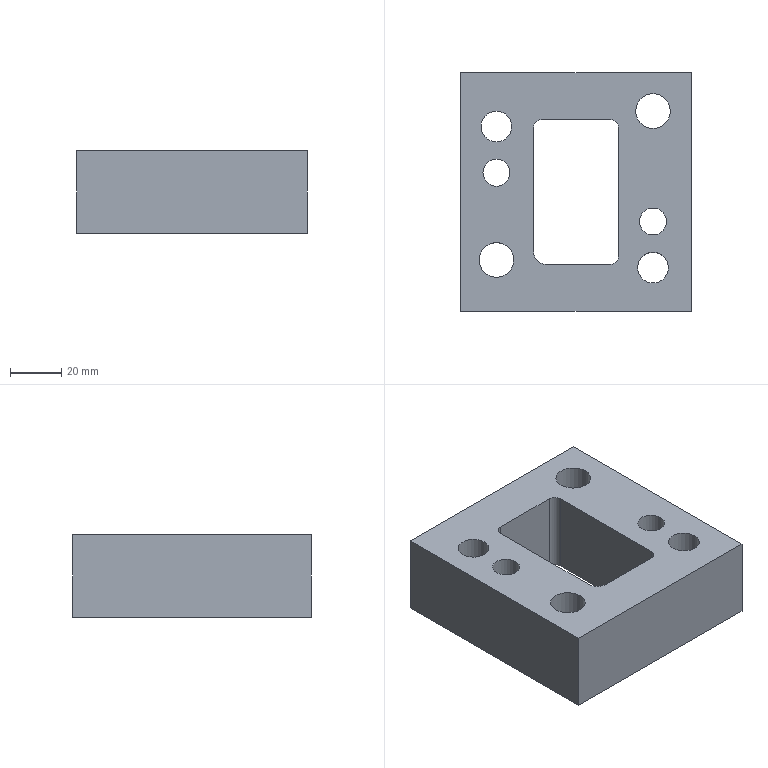Part | STEP file | lll_id2670_x_t | 1 solid | 24 faces | box 90 x 93 x 32 mm | volume 181442 mm3 | plane 12 | cylinder 12 | commonest cylinder face diameters 6 x3 10.505 x2 12 x2 13.509 x2 20.008 x2 10 x1
STEP:
#1=CARTESIAN_POINT('',(472.252,277.75,60.5));
#2=VERTEX_POINT('',#1);
#3=CARTESIAN_POINT('',(467.,277.75,60.5));
#4=DIRECTION('',(0.,0.,1.));
#5=DIRECTION('',(1.,0.,0.));
#6=AXIS2_PLACEMENT_3D('',#3,#4,#5);
#7=CIRCLE('',#6,5.253);
#8=EDGE_CURVE('',#2,#2,#7,.T.);
#9=ORIENTED_EDGE('',*,*,#8,.T.);
#10=EDGE_LOOP('',(#9));
#11=FACE_BOUND('',#10,.T.);
#12=CARTESIAN_POINT('',(395.996,262.75,60.5));
#13=VERTEX_POINT('',#12);
#14=CARTESIAN_POINT('',(406.,262.75,60.5));
#15=DIRECTION('',(0.,0.,1.));
#16=DIRECTION('',(-1.,0.,0.));
#17=AXIS2_PLACEMENT_3D('',#14,#15,#16);
#18=CIRCLE('',#17,10.004);
#19=EDGE_CURVE('',#13,#13,#18,.T.);
#20=ORIENTED_EDGE('',*,*,#19,.T.);
#21=EDGE_LOOP('',(#20));
#22=FACE_BOUND('',#21,.T.);
#23=CARTESIAN_POINT('',(420.5,314.5,60.5));
#24=VERTEX_POINT('',#23);
#25=CARTESIAN_POINT('',(420.5,266.,60.5));
#26=VERTEX_POINT('',#25);
#27=CARTESIAN_POINT('',(420.5,300.,60.5));
#28=DIRECTION('',(0.,-1.,0.));
#29=VECTOR('',#28,1.);
#30=LINE('',#27,#29);
#31=EDGE_CURVE('',#24,#26,#30,.T.);
#32=ORIENTED_EDGE('',*,*,#31,.T.);
#33=CARTESIAN_POINT('',(425.5,261.,60.5));
#34=VERTEX_POINT('',#33);
#35=CARTESIAN_POINT('',(425.5,266.,60.5));
#36=DIRECTION('',(0.,0.,1.));
#37=DIRECTION('',(-1.,0.,0.));
#38=AXIS2_PLACEMENT_3D('',#35,#36,#37);
#39=CIRCLE('',#38,5.);
#40=EDGE_CURVE('',#26,#34,#39,.T.);
#41=ORIENTED_EDGE('',*,*,#40,.T.);
#42=CARTESIAN_POINT('',(450.5,261.,60.5));
#43=VERTEX_POINT('',#42);
#44=CARTESIAN_POINT('',(437.,261.,60.5));
#45=DIRECTION('',(1.,0.,0.));
#46=VECTOR('',#45,1.);
#47=LINE('',#44,#46);
#48=EDGE_CURVE('',#34,#43,#47,.T.);
#49=ORIENTED_EDGE('',*,*,#48,.T.);
#50=CARTESIAN_POINT('',(453.5,264.,60.5));
#51=VERTEX_POINT('',#50);
#52=CARTESIAN_POINT('',(450.5,264.,60.5));
#53=DIRECTION('',(0.,0.,1.));
#54=DIRECTION('',(-1.,0.,0.));
#55=AXIS2_PLACEMENT_3D('',#52,#53,#54);
#56=CIRCLE('',#55,3.);
#57=EDGE_CURVE('',#43,#51,#56,.T.);
#58=ORIENTED_EDGE('',*,*,#57,.T.);
#59=CARTESIAN_POINT('',(453.5,314.5,60.5));
#60=VERTEX_POINT('',#59);
#61=CARTESIAN_POINT('',(453.5,300.,60.5));
#62=DIRECTION('',(0.,1.,0.));
#63=VECTOR('',#62,1.);
#64=LINE('',#61,#63);
#65=EDGE_CURVE('',#51,#60,#64,.T.);
#66=ORIENTED_EDGE('',*,*,#65,.T.);
#67=CARTESIAN_POINT('',(450.5,317.5,60.5));
#68=VERTEX_POINT('',#67);
#69=CARTESIAN_POINT('',(450.5,314.5,60.5));
#70=DIRECTION('',(0.,0.,1.));
#71=DIRECTION('',(-1.,0.,0.));
#72=AXIS2_PLACEMENT_3D('',#69,#70,#71);
#73=CIRCLE('',#72,3.);
#74=EDGE_CURVE('',#60,#68,#73,.T.);
#75=ORIENTED_EDGE('',*,*,#74,.T.);
#76=CARTESIAN_POINT('',(423.5,317.5,60.5));
#77=VERTEX_POINT('',#76);
#78=CARTESIAN_POINT('',(437.,317.5,60.5));
#79=DIRECTION('',(-1.,0.,0.));
#80=VECTOR('',#79,1.);
#81=LINE('',#78,#80);
#82=EDGE_CURVE('',#68,#77,#81,.T.);
#83=ORIENTED_EDGE('',*,*,#82,.T.);
#84=CARTESIAN_POINT('',(423.5,314.5,60.5));
#85=DIRECTION('',(0.,0.,1.));
#86=DIRECTION('',(-1.,0.,0.));
#87=AXIS2_PLACEMENT_3D('',#84,#85,#86);
#88=CIRCLE('',#87,3.);
#89=EDGE_CURVE('',#77,#24,#88,.T.);
#90=ORIENTED_EDGE('',*,*,#89,.T.);
#91=EDGE_LOOP('',(#32,#41,#49,#58,#66,#75,#83,#90));
#92=FACE_BOUND('',#91,.T.);
#93=CARTESIAN_POINT('',(392.,335.75,60.5));
#94=VERTEX_POINT('',#93);
#95=CARTESIAN_POINT('',(392.,242.75,60.5));
#96=VERTEX_POINT('',#95);
#97=CARTESIAN_POINT('',(392.,291.75,60.5));
#98=DIRECTION('',(0.,-1.,0.));
#99=VECTOR('',#98,1.);
#100=LINE('',#97,#99);
#101=EDGE_CURVE('',#94,#96,#100,.T.);
#102=ORIENTED_EDGE('',*,*,#101,.F.);
#103=CARTESIAN_POINT('',(482.,335.75,60.5));
#104=VERTEX_POINT('',#103);
#105=CARTESIAN_POINT('',(437.,335.75,60.5));
#106=DIRECTION('',(-1.,0.,0.));
#107=VECTOR('',#106,1.);
#108=LINE('',#105,#107);
#109=EDGE_CURVE('',#104,#94,#108,.T.);
#110=ORIENTED_EDGE('',*,*,#109,.F.);
#111=CARTESIAN_POINT('',(482.,242.75,60.5));
#112=VERTEX_POINT('',#111);
#113=CARTESIAN_POINT('',(482.,291.75,60.5));
#114=DIRECTION('',(0.,1.,0.));
#115=VECTOR('',#114,1.);
#116=LINE('',#113,#115);
#117=EDGE_CURVE('',#112,#104,#116,.T.);
#118=ORIENTED_EDGE('',*,*,#117,.F.);
#119=CARTESIAN_POINT('',(437.,242.75,60.5));
#120=DIRECTION('',(1.,0.,0.));
#121=VECTOR('',#120,1.);
#122=LINE('',#119,#121);
#123=EDGE_CURVE('',#96,#112,#122,.T.);
#124=ORIENTED_EDGE('',*,*,#123,.F.);
#125=EDGE_LOOP('',(#102,#110,#118,#124));
#126=FACE_BOUND('',#125,.T.);
#127=CARTESIAN_POINT('',(412.,314.75,60.5));
#128=VERTEX_POINT('',#127);
#129=CARTESIAN_POINT('',(406.,314.75,60.5));
#130=DIRECTION('',(0.,0.,-1.));
#131=DIRECTION('',(1.,0.,0.));
#132=AXIS2_PLACEMENT_3D('',#129,#130,#131);
#133=CIRCLE('',#132,6.);
#134=EDGE_CURVE('',#128,#128,#133,.T.);
#135=ORIENTED_EDGE('',*,*,#134,.F.);
#136=EDGE_LOOP('',(#135));
#137=FACE_BOUND('',#136,.T.);
#138=CARTESIAN_POINT('',(461.,259.75,60.5));
#139=VERTEX_POINT('',#138);
#140=CARTESIAN_POINT('',(467.,259.75,60.5));
#141=DIRECTION('',(0.,0.,-1.));
#142=DIRECTION('',(-1.,0.,0.));
#143=AXIS2_PLACEMENT_3D('',#140,#141,#142);
#144=CIRCLE('',#143,6.);
#145=EDGE_CURVE('',#139,#139,#144,.T.);
#146=ORIENTED_EDGE('',*,*,#145,.F.);
#147=EDGE_LOOP('',(#146));
#148=FACE_BOUND('',#147,.T.);
#149=CARTESIAN_POINT('',(477.004,320.75,60.5));
#150=VERTEX_POINT('',#149);
#151=CARTESIAN_POINT('',(467.,320.75,60.5));
#152=DIRECTION('',(0.,0.,1.));
#153=DIRECTION('',(1.,0.,0.));
#154=AXIS2_PLACEMENT_3D('',#151,#152,#153);
#155=CIRCLE('',#154,10.004);
#156=EDGE_CURVE('',#150,#150,#155,.T.);
#157=ORIENTED_EDGE('',*,*,#156,.T.);
#158=EDGE_LOOP('',(#157));
#159=FACE_BOUND('',#158,.T.);
#160=CARTESIAN_POINT('',(411.252,296.75,60.5));
#161=VERTEX_POINT('',#160);
#162=CARTESIAN_POINT('',(406.,296.75,60.5));
#163=DIRECTION('',(0.,0.,1.));
#164=DIRECTION('',(1.,0.,0.));
#165=AXIS2_PLACEMENT_3D('',#162,#163,#164);
#166=CIRCLE('',#165,5.253);
#167=EDGE_CURVE('',#161,#161,#166,.T.);
#168=ORIENTED_EDGE('',*,*,#167,.T.);
#169=EDGE_LOOP('',(#168));
#170=FACE_BOUND('',#169,.T.);
#171=CARTESIAN_POINT('',(437.,291.75,60.5));
#172=DIRECTION('',(0.,0.,-1.));
#173=DIRECTION('',(1.,0.,0.));
#174=AXIS2_PLACEMENT_3D('',#171,#172,#173);
#175=PLANE('',#174);
#176=ADVANCED_FACE('',(#11,#22,#92,#126,#137,#148,#159,#170),#175,.T.);
#177=CARTESIAN_POINT('',(411.252,296.75,92.5));
#178=VERTEX_POINT('',#177);
#179=CARTESIAN_POINT('',(406.,296.75,92.5));
#180=DIRECTION('',(0.,0.,1.));
#181=DIRECTION('',(1.,0.,0.));
#182=AXIS2_PLACEMENT_3D('',#179,#180,#181);
#183=CIRCLE('',#182,5.253);
#184=EDGE_CURVE('',#178,#178,#183,.T.);
#185=ORIENTED_EDGE('',*,*,#184,.F.);
#186=EDGE_LOOP('',(#185));
#187=FACE_BOUND('',#186,.T.);
#188=CARTESIAN_POINT('',(472.252,277.75,92.5));
#189=VERTEX_POINT('',#188);
#190=CARTESIAN_POINT('',(467.,277.75,92.5));
#191=DIRECTION('',(0.,0.,1.));
#192=DIRECTION('',(1.,0.,0.));
#193=AXIS2_PLACEMENT_3D('',#190,#191,#192);
#194=CIRCLE('',#193,5.253);
#195=EDGE_CURVE('',#189,#189,#194,.T.);
#196=ORIENTED_EDGE('',*,*,#195,.F.);
#197=EDGE_LOOP('',(#196));
#198=FACE_BOUND('',#197,.T.);
#199=CARTESIAN_POINT('',(460.245,320.75,92.5));
#200=VERTEX_POINT('',#199);
#201=CARTESIAN_POINT('',(467.,320.75,92.5));
#202=DIRECTION('',(0.,0.,1.));
#203=DIRECTION('',(-1.,0.,0.));
#204=AXIS2_PLACEMENT_3D('',#201,#202,#203);
#205=CIRCLE('',#204,6.755);
#206=EDGE_CURVE('',#200,#200,#205,.T.);
#207=ORIENTED_EDGE('',*,*,#206,.F.);
#208=EDGE_LOOP('',(#207));
#209=FACE_BOUND('',#208,.T.);
#210=CARTESIAN_POINT('',(399.245,262.75,92.5));
#211=VERTEX_POINT('',#210);
#212=CARTESIAN_POINT('',(406.,262.75,92.5));
#213=DIRECTION('',(0.,0.,1.));
#214=DIRECTION('',(-1.,0.,0.));
#215=AXIS2_PLACEMENT_3D('',#212,#213,#214);
#216=CIRCLE('',#215,6.755);
#217=EDGE_CURVE('',#211,#211,#216,.T.);
#218=ORIENTED_EDGE('',*,*,#217,.F.);
#219=EDGE_LOOP('',(#218));
#220=FACE_BOUND('',#219,.T.);
#221=CARTESIAN_POINT('',(453.5,314.5,92.5));
#222=VERTEX_POINT('',#221);
#223=CARTESIAN_POINT('',(453.5,264.,92.5));
#224=VERTEX_POINT('',#223);
#225=CARTESIAN_POINT('',(453.5,300.,92.5));
#226=DIRECTION('',(0.,-1.,0.));
#227=VECTOR('',#226,1.);
#228=LINE('',#225,#227);
#229=EDGE_CURVE('',#222,#224,#228,.T.);
#230=ORIENTED_EDGE('',*,*,#229,.T.);
#231=CARTESIAN_POINT('',(450.5,261.,92.5));
#232=VERTEX_POINT('',#231);
#233=CARTESIAN_POINT('',(450.5,264.,92.5));
#234=DIRECTION('',(0.,0.,-1.));
#235=DIRECTION('',(1.,0.,0.));
#236=AXIS2_PLACEMENT_3D('',#233,#234,#235);
#237=CIRCLE('',#236,3.);
#238=EDGE_CURVE('',#224,#232,#237,.T.);
#239=ORIENTED_EDGE('',*,*,#238,.T.);
#240=CARTESIAN_POINT('',(425.5,261.,92.5));
#241=VERTEX_POINT('',#240);
#242=CARTESIAN_POINT('',(437.,261.,92.5));
#243=DIRECTION('',(-1.,0.,0.));
#244=VECTOR('',#243,1.);
#245=LINE('',#242,#244);
#246=EDGE_CURVE('',#232,#241,#245,.T.);
#247=ORIENTED_EDGE('',*,*,#246,.T.);
#248=CARTESIAN_POINT('',(420.5,266.,92.5));
#249=VERTEX_POINT('',#248);
#250=CARTESIAN_POINT('',(425.5,266.,92.5));
#251=DIRECTION('',(0.,0.,-1.));
#252=DIRECTION('',(1.,0.,0.));
#253=AXIS2_PLACEMENT_3D('',#250,#251,#252);
#254=CIRCLE('',#253,5.);
#255=EDGE_CURVE('',#241,#249,#254,.T.);
#256=ORIENTED_EDGE('',*,*,#255,.T.);
#257=CARTESIAN_POINT('',(420.5,314.5,92.5));
#258=VERTEX_POINT('',#257);
#259=CARTESIAN_POINT('',(420.5,300.,92.5));
#260=DIRECTION('',(0.,1.,0.));
#261=VECTOR('',#260,1.);
#262=LINE('',#259,#261);
#263=EDGE_CURVE('',#249,#258,#262,.T.);
#264=ORIENTED_EDGE('',*,*,#263,.T.);
#265=CARTESIAN_POINT('',(423.5,317.5,92.5));
#266=VERTEX_POINT('',#265);
#267=CARTESIAN_POINT('',(423.5,314.5,92.5));
#268=DIRECTION('',(0.,0.,-1.));
#269=DIRECTION('',(1.,0.,0.));
#270=AXIS2_PLACEMENT_3D('',#267,#268,#269);
#271=CIRCLE('',#270,3.);
#272=EDGE_CURVE('',#258,#266,#271,.T.);
#273=ORIENTED_EDGE('',*,*,#272,.T.);
#274=CARTESIAN_POINT('',(450.5,317.5,92.5));
#275=VERTEX_POINT('',#274);
#276=CARTESIAN_POINT('',(437.,317.5,92.5));
#277=DIRECTION('',(1.,0.,0.));
#278=VECTOR('',#277,1.);
#279=LINE('',#276,#278);
#280=EDGE_CURVE('',#266,#275,#279,.T.);
#281=ORIENTED_EDGE('',*,*,#280,.T.);
#282=CARTESIAN_POINT('',(450.5,314.5,92.5));
#283=DIRECTION('',(0.,0.,-1.));
#284=DIRECTION('',(1.,0.,0.));
#285=AXIS2_PLACEMENT_3D('',#282,#283,#284);
#286=CIRCLE('',#285,3.);
#287=EDGE_CURVE('',#275,#222,#286,.T.);
#288=ORIENTED_EDGE('',*,*,#287,.T.);
#289=EDGE_LOOP('',(#230,#239,#247,#256,#264,#273,#281,#288));
#290=FACE_BOUND('',#289,.T.);
#291=CARTESIAN_POINT('',(392.,335.75,92.5));
#292=VERTEX_POINT('',#291);
#293=CARTESIAN_POINT('',(482.,335.75,92.5));
#294=VERTEX_POINT('',#293);
#295=CARTESIAN_POINT('',(437.,335.75,92.5));
#296=DIRECTION('',(1.,0.,0.));
#297=VECTOR('',#296,1.);
#298=LINE('',#295,#297);
#299=EDGE_CURVE('',#292,#294,#298,.T.);
#300=ORIENTED_EDGE('',*,*,#299,.F.);
#301=CARTESIAN_POINT('',(392.,242.75,92.5));
#302=VERTEX_POINT('',#301);
#303=CARTESIAN_POINT('',(392.,291.75,92.5));
#304=DIRECTION('',(0.,1.,0.));
#305=VECTOR('',#304,1.);
#306=LINE('',#303,#305);
#307=EDGE_CURVE('',#302,#292,#306,.T.);
#308=ORIENTED_EDGE('',*,*,#307,.F.);
#309=CARTESIAN_POINT('',(482.,242.75,92.5));
#310=VERTEX_POINT('',#309);
#311=CARTESIAN_POINT('',(437.,242.75,92.5));
#312=DIRECTION('',(-1.,0.,0.));
#313=VECTOR('',#312,1.);
#314=LINE('',#311,#313);
#315=EDGE_CURVE('',#310,#302,#314,.T.);
#316=ORIENTED_EDGE('',*,*,#315,.F.);
#317=CARTESIAN_POINT('',(482.,291.75,92.5));
#318=DIRECTION('',(0.,-1.,0.));
#319=VECTOR('',#318,1.);
#320=LINE('',#317,#319);
#321=EDGE_CURVE('',#294,#310,#320,.T.);
#322=ORIENTED_EDGE('',*,*,#321,.F.);
#323=EDGE_LOOP('',(#300,#308,#316,#322));
#324=FACE_BOUND('',#323,.T.);
#325=CARTESIAN_POINT('',(400.,314.75,92.5));
#326=VERTEX_POINT('',#325);
#327=CARTESIAN_POINT('',(406.,314.75,92.5));
#328=DIRECTION('',(0.,0.,-1.));
#329=DIRECTION('',(-1.,0.,0.));
#330=AXIS2_PLACEMENT_3D('',#327,#328,#329);
#331=CIRCLE('',#330,6.);
#332=EDGE_CURVE('',#326,#326,#331,.T.);
#333=ORIENTED_EDGE('',*,*,#332,.T.);
#334=EDGE_LOOP('',(#333));
#335=FACE_BOUND('',#334,.T.);
#336=CARTESIAN_POINT('',(473.,259.75,92.5));
#337=VERTEX_POINT('',#336);
#338=CARTESIAN_POINT('',(467.,259.75,92.5));
#339=DIRECTION('',(0.,0.,-1.));
#340=DIRECTION('',(1.,0.,0.));
#341=AXIS2_PLACEMENT_3D('',#338,#339,#340);
#342=CIRCLE('',#341,6.);
#343=EDGE_CURVE('',#337,#337,#342,.T.);
#344=ORIENTED_EDGE('',*,*,#343,.T.);
#345=EDGE_LOOP('',(#344));
#346=FACE_BOUND('',#345,.T.);
#347=CARTESIAN_POINT('',(437.,291.75,92.5));
#348=DIRECTION('',(0.,0.,1.));
#349=DIRECTION('',(-1.,0.,0.));
#350=AXIS2_PLACEMENT_3D('',#347,#348,#349);
#351=PLANE('',#350);
#352=ADVANCED_FACE('',(#187,#198,#209,#220,#290,#324,#335,#346),#351,.T.);
#353=CARTESIAN_POINT('',(392.,335.75,60.5));
#354=DIRECTION('',(0.,0.,1.));
#355=VECTOR('',#354,1.);
#356=LINE('',#353,#355);
#357=EDGE_CURVE('',#94,#292,#356,.T.);
#358=ORIENTED_EDGE('',*,*,#357,.T.);
#359=ORIENTED_EDGE('',*,*,#299,.T.);
#360=CARTESIAN_POINT('',(482.,335.75,60.5));
#361=DIRECTION('',(0.,0.,1.));
#362=VECTOR('',#361,1.);
#363=LINE('',#360,#362);
#364=EDGE_CURVE('',#104,#294,#363,.T.);
#365=ORIENTED_EDGE('',*,*,#364,.F.);
#366=ORIENTED_EDGE('',*,*,#109,.T.);
#367=EDGE_LOOP('',(#358,#359,#365,#366));
#368=FACE_OUTER_BOUND('',#367,.T.);
#369=CARTESIAN_POINT('',(437.,335.75,60.5));
#370=DIRECTION('',(0.,1.,0.));
#371=DIRECTION('',(0.,0.,-1.));
#372=AXIS2_PLACEMENT_3D('',#369,#370,#371);
#373=PLANE('',#372);
#374=ADVANCED_FACE('',(#368),#373,.T.);
#375=ORIENTED_EDGE('',*,*,#364,.T.);
#376=ORIENTED_EDGE('',*,*,#321,.T.);
#377=CARTESIAN_POINT('',(482.,242.75,60.5));
#378=DIRECTION('',(0.,0.,1.));
#379=VECTOR('',#378,1.);
#380=LINE('',#377,#379);
#381=EDGE_CURVE('',#112,#310,#380,.T.);
#382=ORIENTED_EDGE('',*,*,#381,.F.);
#383=ORIENTED_EDGE('',*,*,#117,.T.);
#384=EDGE_LOOP('',(#375,#376,#382,#383));
#385=FACE_OUTER_BOUND('',#384,.T.);
#386=CARTESIAN_POINT('',(482.,291.75,60.5));
#387=DIRECTION('',(1.,0.,0.));
#388=DIRECTION('',(0.,0.,1.));
#389=AXIS2_PLACEMENT_3D('',#386,#387,#388);
#390=PLANE('',#389);
#391=ADVANCED_FACE('',(#385),#390,.T.);
#392=ORIENTED_EDGE('',*,*,#381,.T.);
#393=ORIENTED_EDGE('',*,*,#315,.T.);
#394=CARTESIAN_POINT('',(392.,242.75,60.5));
#395=DIRECTION('',(0.,0.,1.));
#396=VECTOR('',#395,1.);
#397=LINE('',#394,#396);
#398=EDGE_CURVE('',#96,#302,#397,.T.);
#399=ORIENTED_EDGE('',*,*,#398,.F.);
#400=ORIENTED_EDGE('',*,*,#123,.T.);
#401=EDGE_LOOP('',(#392,#393,#399,#400));
#402=FACE_OUTER_BOUND('',#401,.T.);
#403=CARTESIAN_POINT('',(437.,242.75,60.5));
#404=DIRECTION('',(0.,-1.,0.));
#405=DIRECTION('',(0.,0.,1.));
#406=AXIS2_PLACEMENT_3D('',#403,#404,#405);
#407=PLANE('',#406);
#408=ADVANCED_FACE('',(#402),#407,.T.);
#409=ORIENTED_EDGE('',*,*,#101,.T.);
#410=ORIENTED_EDGE('',*,*,#398,.T.);
#411=ORIENTED_EDGE('',*,*,#307,.T.);
#412=ORIENTED_EDGE('',*,*,#357,.F.);
#413=EDGE_LOOP('',(#409,#410,#411,#412));
#414=FACE_OUTER_BOUND('',#413,.T.);
#415=CARTESIAN_POINT('',(392.,291.75,60.5));
#416=DIRECTION('',(-1.,0.,0.));
#417=DIRECTION('',(0.,0.,-1.));
#418=AXIS2_PLACEMENT_3D('',#415,#416,#417);
#419=PLANE('',#418);
#420=ADVANCED_FACE('',(#414),#419,.T.);
#421=ORIENTED_EDGE('',*,*,#65,.F.);
#422=CARTESIAN_POINT('',(453.5,264.,92.5));
#423=DIRECTION('',(0.,0.,1.));
#424=VECTOR('',#423,1.);
#425=LINE('',#422,#424);
#426=EDGE_CURVE('',#51,#224,#425,.T.);
#427=ORIENTED_EDGE('',*,*,#426,.T.);
#428=ORIENTED_EDGE('',*,*,#229,.F.);
#429=CARTESIAN_POINT('',(453.5,314.5,60.5));
#430=DIRECTION('',(0.,0.,-1.));
#431=VECTOR('',#430,1.);
#432=LINE('',#429,#431);
#433=EDGE_CURVE('',#222,#60,#432,.T.);
#434=ORIENTED_EDGE('',*,*,#433,.T.);
#435=EDGE_LOOP('',(#421,#427,#428,#434));
#436=FACE_OUTER_BOUND('',#435,.T.);
#437=CARTESIAN_POINT('',(453.5,300.,-8.5));
#438=DIRECTION('',(1.,0.,0.));
#439=DIRECTION('',(0.,0.,1.));
#440=AXIS2_PLACEMENT_3D('',#437,#438,#439);
#441=PLANE('',#440);
#442=ADVANCED_FACE('',(#436),#441,.F.);
#443=ORIENTED_EDGE('',*,*,#48,.F.);
#444=CARTESIAN_POINT('',(425.5,261.,92.5));
#445=DIRECTION('',(0.,0.,1.));
#446=VECTOR('',#445,1.);
#447=LINE('',#444,#446);
#448=EDGE_CURVE('',#34,#241,#447,.T.);
#449=ORIENTED_EDGE('',*,*,#448,.T.);
#450=ORIENTED_EDGE('',*,*,#246,.F.);
#451=CARTESIAN_POINT('',(450.5,261.,60.5));
#452=DIRECTION('',(0.,0.,-1.));
#453=VECTOR('',#452,1.);
#454=LINE('',#451,#453);
#455=EDGE_CURVE('',#232,#43,#454,.T.);
#456=ORIENTED_EDGE('',*,*,#455,.T.);
#457=EDGE_LOOP('',(#443,#449,#450,#456));
#458=FACE_OUTER_BOUND('',#457,.T.);
#459=CARTESIAN_POINT('',(437.,261.,-8.5));
#460=DIRECTION('',(0.,-1.,0.));
#461=DIRECTION('',(0.,0.,1.));
#462=AXIS2_PLACEMENT_3D('',#459,#460,#461);
#463=PLANE('',#462);
#464=ADVANCED_FACE('',(#458),#463,.F.);
#465=ORIENTED_EDGE('',*,*,#263,.F.);
#466=CARTESIAN_POINT('',(420.5,266.,60.5));
#467=DIRECTION('',(0.,0.,-1.));
#468=VECTOR('',#467,1.);
#469=LINE('',#466,#468);
#470=EDGE_CURVE('',#249,#26,#469,.T.);
#471=ORIENTED_EDGE('',*,*,#470,.T.);
#472=ORIENTED_EDGE('',*,*,#31,.F.);
#473=CARTESIAN_POINT('',(420.5,314.5,92.5));
#474=DIRECTION('',(0.,0.,1.));
#475=VECTOR('',#474,1.);
#476=LINE('',#473,#475);
#477=EDGE_CURVE('',#24,#258,#476,.T.);
#478=ORIENTED_EDGE('',*,*,#477,.T.);
#479=EDGE_LOOP('',(#465,#471,#472,#478));
#480=FACE_OUTER_BOUND('',#479,.T.);
#481=CARTESIAN_POINT('',(420.5,300.,-8.5));
#482=DIRECTION('',(-1.,0.,0.));
#483=DIRECTION('',(0.,0.,-1.));
#484=AXIS2_PLACEMENT_3D('',#481,#482,#483);
#485=PLANE('',#484);
#486=ADVANCED_FACE('',(#480),#485,.F.);
#487=ORIENTED_EDGE('',*,*,#82,.F.);
#488=CARTESIAN_POINT('',(450.5,317.5,92.5));
#489=DIRECTION('',(0.,0.,1.));
#490=VECTOR('',#489,1.);
#491=LINE('',#488,#490);
#492=EDGE_CURVE('',#68,#275,#491,.T.);
#493=ORIENTED_EDGE('',*,*,#492,.T.);
#494=ORIENTED_EDGE('',*,*,#280,.F.);
#495=CARTESIAN_POINT('',(423.5,317.5,60.5));
#496=DIRECTION('',(0.,0.,-1.));
#497=VECTOR('',#496,1.);
#498=LINE('',#495,#497);
#499=EDGE_CURVE('',#266,#77,#498,.T.);
#500=ORIENTED_EDGE('',*,*,#499,.T.);
#501=EDGE_LOOP('',(#487,#493,#494,#500));
#502=FACE_OUTER_BOUND('',#501,.T.);
#503=CARTESIAN_POINT('',(437.,317.5,-8.5));
#504=DIRECTION('',(0.,1.,0.));
#505=DIRECTION('',(0.,0.,-1.));
#506=AXIS2_PLACEMENT_3D('',#503,#504,#505);
#507=PLANE('',#506);
#508=ADVANCED_FACE('',(#502),#507,.F.);
#509=CARTESIAN_POINT('',(395.996,262.75,75.5));
#510=VERTEX_POINT('',#509);
#511=CARTESIAN_POINT('',(406.,262.75,75.5));
#512=DIRECTION('',(0.,0.,1.));
#513=DIRECTION('',(-1.,0.,0.));
#514=AXIS2_PLACEMENT_3D('',#511,#512,#513);
#515=CIRCLE('',#514,10.004);
#516=EDGE_CURVE('',#510,#510,#515,.T.);
#517=ORIENTED_EDGE('',*,*,#516,.T.);
#518=EDGE_LOOP('',(#517));
#519=FACE_BOUND('',#518,.T.);
#520=ORIENTED_EDGE('',*,*,#19,.F.);
#521=EDGE_LOOP('',(#520));
#522=FACE_BOUND('',#521,.T.);
#523=CARTESIAN_POINT('',(406.,262.75,60.5));
#524=DIRECTION('',(0.,0.,1.));
#525=DIRECTION('',(-1.,0.,0.));
#526=AXIS2_PLACEMENT_3D('',#523,#524,#525);
#527=CYLINDRICAL_SURFACE('',#526,10.004);
#528=ADVANCED_FACE('',(#519,#522),#527,.F.);
#529=ORIENTED_EDGE('',*,*,#217,.T.);
#530=EDGE_LOOP('',(#529));
#531=FACE_BOUND('',#530,.T.);
#532=CARTESIAN_POINT('',(399.245,262.75,75.5));
#533=VERTEX_POINT('',#532);
#534=CARTESIAN_POINT('',(406.,262.75,75.5));
#535=DIRECTION('',(0.,0.,1.));
#536=DIRECTION('',(-1.,0.,0.));
#537=AXIS2_PLACEMENT_3D('',#534,#535,#536);
#538=CIRCLE('',#537,6.755);
#539=EDGE_CURVE('',#533,#533,#538,.T.);
#540=ORIENTED_EDGE('',*,*,#539,.F.);
#541=EDGE_LOOP('',(#540));
#542=FACE_BOUND('',#541,.T.);
#543=CARTESIAN_POINT('',(406.,262.75,57.5));
#544=DIRECTION('',(0.,0.,1.));
#545=DIRECTION('',(-1.,0.,0.));
#546=AXIS2_PLACEMENT_3D('',#543,#544,#545);
#547=CYLINDRICAL_SURFACE('',#546,6.755);
#548=ADVANCED_FACE('',(#531,#542),#547,.F.);
#549=ORIENTED_EDGE('',*,*,#539,.T.);
#550=EDGE_LOOP('',(#549));
#551=FACE_BOUND('',#550,.T.);
#552=ORIENTED_EDGE('',*,*,#516,.F.);
#553=EDGE_LOOP('',(#552));
#554=FACE_BOUND('',#553,.T.);
#555=CARTESIAN_POINT('',(406.,262.75,75.5));
#556=DIRECTION('',(0.,0.,1.));
#557=DIRECTION('',(-1.,0.,0.));
#558=AXIS2_PLACEMENT_3D('',#555,#556,#557);
#559=PLANE('',#558);
#560=ADVANCED_FACE('',(#551,#554),#559,.F.);
#561=ORIENTED_EDGE('',*,*,#134,.T.);
#562=EDGE_LOOP('',(#561));
#563=FACE_BOUND('',#562,.T.);
#564=ORIENTED_EDGE('',*,*,#332,.F.);
#565=EDGE_LOOP('',(#564));
#566=FACE_BOUND('',#565,.T.);
#567=CARTESIAN_POINT('',(406.,314.75,57.5));
#568=DIRECTION('',(0.,0.,1.));
#569=DIRECTION('',(-1.,0.,0.));
#570=AXIS2_PLACEMENT_3D('',#567,#568,#569);
#571=CYLINDRICAL_SURFACE('',#570,6.);
#572=ADVANCED_FACE('',(#563,#566),#571,.F.);
#573=ORIENTED_EDGE('',*,*,#145,.T.);
#574=EDGE_LOOP('',(#573));
#575=FACE_BOUND('',#574,.T.);
#576=ORIENTED_EDGE('',*,*,#343,.F.);
#577=EDGE_LOOP('',(#576));
#578=FACE_BOUND('',#577,.T.);
#579=CARTESIAN_POINT('',(467.,259.75,57.5));
#580=DIRECTION('',(0.,0.,1.));
#581=DIRECTION('',(1.,0.,0.));
#582=AXIS2_PLACEMENT_3D('',#579,#580,#581);
#583=CYLINDRICAL_SURFACE('',#582,6.);
#584=ADVANCED_FACE('',(#575,#578),#583,.F.);
#585=CARTESIAN_POINT('',(477.004,320.75,75.5));
#586=VERTEX_POINT('',#585);
#587=CARTESIAN_POINT('',(467.,320.75,75.5));
#588=DIRECTION('',(0.,0.,1.));
#589=DIRECTION('',(1.,0.,0.));
#590=AXIS2_PLACEMENT_3D('',#587,#588,#589);
#591=CIRCLE('',#590,10.004);
#592=EDGE_CURVE('',#586,#586,#591,.T.);
#593=ORIENTED_EDGE('',*,*,#592,.T.);
#594=EDGE_LOOP('',(#593));
#595=FACE_BOUND('',#594,.T.);
#596=ORIENTED_EDGE('',*,*,#156,.F.);
#597=EDGE_LOOP('',(#596));
#598=FACE_BOUND('',#597,.T.);
#599=CARTESIAN_POINT('',(467.,320.75,60.5));
#600=DIRECTION('',(0.,0.,1.));
#601=DIRECTION('',(1.,0.,0.));
#602=AXIS2_PLACEMENT_3D('',#599,#600,#601);
#603=CYLINDRICAL_SURFACE('',#602,10.004);
#604=ADVANCED_FACE('',(#595,#598),#603,.F.);
#605=ORIENTED_EDGE('',*,*,#206,.T.);
#606=EDGE_LOOP('',(#605));
#607=FACE_BOUND('',#606,.T.);
#608=CARTESIAN_POINT('',(473.754,320.75,75.5));
#609=VERTEX_POINT('',#608);
#610=CARTESIAN_POINT('',(467.,320.75,75.5));
#611=DIRECTION('',(0.,0.,1.));
#612=DIRECTION('',(1.,0.,0.));
#613=AXIS2_PLACEMENT_3D('',#610,#611,#612);
#614=CIRCLE('',#613,6.755);
#615=EDGE_CURVE('',#609,#609,#614,.T.);
#616=ORIENTED_EDGE('',*,*,#615,.F.);
#617=EDGE_LOOP('',(#616));
#618=FACE_BOUND('',#617,.T.);
#619=CARTESIAN_POINT('',(467.,320.75,57.5));
#620=DIRECTION('',(0.,0.,1.));
#621=DIRECTION('',(1.,0.,0.));
#622=AXIS2_PLACEMENT_3D('',#619,#620,#621);
#623=CYLINDRICAL_SURFACE('',#622,6.755);
#624=ADVANCED_FACE('',(#607,#618),#623,.F.);
#625=ORIENTED_EDGE('',*,*,#615,.T.);
#626=EDGE_LOOP('',(#625));
#627=FACE_BOUND('',#626,.T.);
#628=ORIENTED_EDGE('',*,*,#592,.F.);
#629=EDGE_LOOP('',(#628));
#630=FACE_BOUND('',#629,.T.);
#631=CARTESIAN_POINT('',(467.,320.75,75.5));
#632=DIRECTION('',(0.,0.,1.));
#633=DIRECTION('',(1.,0.,0.));
#634=AXIS2_PLACEMENT_3D('',#631,#632,#633);
#635=PLANE('',#634);
#636=ADVANCED_FACE('',(#627,#630),#635,.F.);
#637=ORIENTED_EDGE('',*,*,#74,.F.);
#638=ORIENTED_EDGE('',*,*,#433,.F.);
#639=ORIENTED_EDGE('',*,*,#287,.F.);
#640=ORIENTED_EDGE('',*,*,#492,.F.);
#641=EDGE_LOOP('',(#637,#638,#639,#640));
#642=FACE_OUTER_BOUND('',#641,.T.);
#643=CARTESIAN_POINT('',(450.5,314.5,-8.5));
#644=DIRECTION('',(0.,0.,-1.));
#645=DIRECTION('',(-1.,0.,0.));
#646=AXIS2_PLACEMENT_3D('',#643,#644,#645);
#647=CYLINDRICAL_SURFACE('',#646,3.);
#648=ADVANCED_FACE('',(#642),#647,.F.);
#649=ORIENTED_EDGE('',*,*,#89,.F.);
#650=ORIENTED_EDGE('',*,*,#499,.F.);
#651=ORIENTED_EDGE('',*,*,#272,.F.);
#652=ORIENTED_EDGE('',*,*,#477,.F.);
#653=EDGE_LOOP('',(#649,#650,#651,#652));
#654=FACE_OUTER_BOUND('',#653,.T.);
#655=CARTESIAN_POINT('',(423.5,314.5,-8.5));
#656=DIRECTION('',(0.,0.,-1.));
#657=DIRECTION('',(-1.,0.,0.));
#658=AXIS2_PLACEMENT_3D('',#655,#656,#657);
#659=CYLINDRICAL_SURFACE('',#658,3.);
#660=ADVANCED_FACE('',(#654),#659,.F.);
#661=ORIENTED_EDGE('',*,*,#238,.F.);
#662=ORIENTED_EDGE('',*,*,#426,.F.);
#663=ORIENTED_EDGE('',*,*,#57,.F.);
#664=ORIENTED_EDGE('',*,*,#455,.F.);
#665=EDGE_LOOP('',(#661,#662,#663,#664));
#666=FACE_OUTER_BOUND('',#665,.T.);
#667=CARTESIAN_POINT('',(450.5,264.,-8.5));
#668=DIRECTION('',(0.,0.,1.));
#669=DIRECTION('',(1.,0.,0.));
#670=AXIS2_PLACEMENT_3D('',#667,#668,#669);
#671=CYLINDRICAL_SURFACE('',#670,3.);
#672=ADVANCED_FACE('',(#666),#671,.F.);
#673=ORIENTED_EDGE('',*,*,#255,.F.);
#674=ORIENTED_EDGE('',*,*,#448,.F.);
#675=ORIENTED_EDGE('',*,*,#40,.F.);
#676=ORIENTED_EDGE('',*,*,#470,.F.);
#677=EDGE_LOOP('',(#673,#674,#675,#676));
#678=FACE_OUTER_BOUND('',#677,.T.);
#679=CARTESIAN_POINT('',(425.5,266.,-8.5));
#680=DIRECTION('',(0.,0.,1.));
#681=DIRECTION('',(1.,0.,0.));
#682=AXIS2_PLACEMENT_3D('',#679,#680,#681);
#683=CYLINDRICAL_SURFACE('',#682,5.);
#684=ADVANCED_FACE('',(#678),#683,.F.);
#685=ORIENTED_EDGE('',*,*,#195,.T.);
#686=EDGE_LOOP('',(#685));
#687=FACE_BOUND('',#686,.T.);
#688=ORIENTED_EDGE('',*,*,#8,.F.);
#689=EDGE_LOOP('',(#688));
#690=FACE_BOUND('',#689,.T.);
#691=CARTESIAN_POINT('',(467.,277.75,60.5));
#692=DIRECTION('',(0.,0.,1.));
#693=DIRECTION('',(1.,0.,0.));
#694=AXIS2_PLACEMENT_3D('',#691,#692,#693);
#695=CYLINDRICAL_SURFACE('',#694,5.253);
#696=ADVANCED_FACE('',(#687,#690),#695,.F.);
#697=ORIENTED_EDGE('',*,*,#184,.T.);
#698=EDGE_LOOP('',(#697));
#699=FACE_BOUND('',#698,.T.);
#700=ORIENTED_EDGE('',*,*,#167,.F.);
#701=EDGE_LOOP('',(#700));
#702=FACE_BOUND('',#701,.T.);
#703=CARTESIAN_POINT('',(406.,296.75,60.5));
#704=DIRECTION('',(0.,0.,1.));
#705=DIRECTION('',(1.,0.,0.));
#706=AXIS2_PLACEMENT_3D('',#703,#704,#705);
#707=CYLINDRICAL_SURFACE('',#706,5.253);
#708=ADVANCED_FACE('',(#699,#702),#707,.F.);
#709=CLOSED_SHELL('',(#176,#352,#374,#391,#408,#420,#442,#464,#486,#508,#528,#548,#560,#572,#584,#604,#624,#636,#648,#660,#672,#684,#696,#708));
#710=MANIFOLD_SOLID_BREP('',#709);
#711=(LENGTH_UNIT()NAMED_UNIT(*)SI_UNIT(.MILLI.,.METRE.));
#712=UNCERTAINTY_MEASURE_WITH_UNIT(LENGTH_MEASURE(0.00002),#711,'','');
#713=(NAMED_UNIT(*)PLANE_ANGLE_UNIT()SI_UNIT($,.RADIAN.));
#714=PLANE_ANGLE_MEASURE_WITH_UNIT(PLANE_ANGLE_MEASURE(0.01745),#713);
#715=DIMENSIONAL_EXPONENTS(0.,0.,0.,0.,0.,0.,0.);
#716=(CONVERSION_BASED_UNIT('DEGREE',#714)NAMED_UNIT(#715)PLANE_ANGLE_UNIT());
#717=(NAMED_UNIT(*)SI_UNIT($,.STERADIAN.)SOLID_ANGLE_UNIT());
#718=(GEOMETRIC_REPRESENTATION_CONTEXT(3)GLOBAL_UNCERTAINTY_ASSIGNED_CONTEXT((#712))GLOBAL_UNIT_ASSIGNED_CONTEXT((#711,#716,#717))REPRESENTATION_CONTEXT('',''));
#719=ADVANCED_BREP_SHAPE_REPRESENTATION('',(#710),#718);